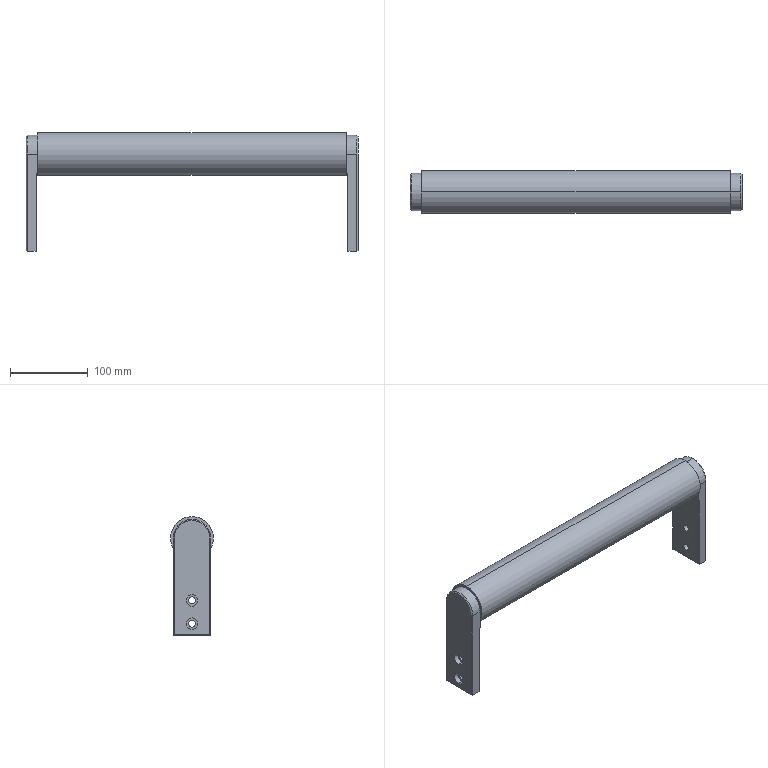Part | SolidWorks | features ICE 2, Chamfer 1, Extrusion 1, HoleWzd 1, MirrorPattern 1 | 1 solid | 54 faces | box 426 x 55 x 152.5 mm | volume 1121917 mm3 | plane 30 | cylinder 21 | cone 3 | commonest cylinder face diameters 9 x8 15 x8 48 x3 55 x2
STEP:
#1=CARTESIAN_POINT('',(-405.,0.,-25.));
#2=VERTEX_POINT('',#1);
#3=CARTESIAN_POINT('',(-405.,0.,-10.));
#4=VERTEX_POINT('',#3);
#5=CARTESIAN_POINT('',(-405.,0.,-17.5));
#6=DIRECTION('',(-1.,0.,0.));
#7=DIRECTION('',(0.,0.,1.));
#8=AXIS2_PLACEMENT_3D('',#5,#6,#7);
#9=CIRCLE('',#8,7.5);
#10=EDGE_CURVE('',#2,#4,#9,.T.);
#11=ORIENTED_EDGE('',*,*,#10,.F.);
#12=CARTESIAN_POINT('',(-411.,0.,-25.));
#13=VERTEX_POINT('',#12);
#14=CARTESIAN_POINT('',(-411.,0.,-25.));
#15=DIRECTION('',(-1.,0.,0.));
#16=VECTOR('',#15,1000.);
#17=LINE('',#14,#16);
#18=EDGE_CURVE('',#2,#13,#17,.T.);
#19=ORIENTED_EDGE('',*,*,#18,.T.);
#20=CARTESIAN_POINT('',(-411.,0.,-10.));
#21=VERTEX_POINT('',#20);
#22=CARTESIAN_POINT('',(-411.,0.,-17.5));
#23=DIRECTION('',(-1.,0.,0.));
#24=DIRECTION('',(0.,0.,1.));
#25=AXIS2_PLACEMENT_3D('',#22,#23,#24);
#26=CIRCLE('',#25,7.5);
#27=EDGE_CURVE('',#13,#21,#26,.T.);
#28=ORIENTED_EDGE('',*,*,#27,.T.);
#29=CARTESIAN_POINT('',(-411.,0.,-10.));
#30=DIRECTION('',(-1.,0.,0.));
#31=VECTOR('',#30,1000.);
#32=LINE('',#29,#31);
#33=EDGE_CURVE('',#4,#21,#32,.T.);
#34=ORIENTED_EDGE('',*,*,#33,.F.);
#35=EDGE_LOOP('',(#11,#19,#28,#34));
#36=FACE_OUTER_BOUND('',#35,.T.);
#37=CARTESIAN_POINT('',(-411.,0.,-17.5));
#38=DIRECTION('',(-1.,0.,0.));
#39=DIRECTION('',(0.,0.,1.));
#40=AXIS2_PLACEMENT_3D('',#37,#38,#39);
#41=CYLINDRICAL_SURFACE('',#40,7.5);
#42=ADVANCED_FACE('',(#36),#41,.F.);
#43=CARTESIAN_POINT('',(-398.,0.,-13.));
#44=VERTEX_POINT('',#43);
#45=CARTESIAN_POINT('',(-398.,0.,-22.));
#46=VERTEX_POINT('',#45);
#47=CARTESIAN_POINT('',(-398.,0.,-17.5));
#48=DIRECTION('',(1.,0.,0.));
#49=DIRECTION('',(0.,0.,1.));
#50=AXIS2_PLACEMENT_3D('',#47,#48,#49);
#51=CIRCLE('',#50,4.5);
#52=EDGE_CURVE('',#44,#46,#51,.T.);
#53=ORIENTED_EDGE('',*,*,#52,.T.);
#54=CARTESIAN_POINT('',(-405.,0.,-22.));
#55=VERTEX_POINT('',#54);
#56=CARTESIAN_POINT('',(-411.,0.,-22.));
#57=DIRECTION('',(-1.,0.,0.));
#58=VECTOR('',#57,1000.);
#59=LINE('',#56,#58);
#60=EDGE_CURVE('',#46,#55,#59,.T.);
#61=ORIENTED_EDGE('',*,*,#60,.T.);
#62=CARTESIAN_POINT('',(-405.,0.,-13.));
#63=VERTEX_POINT('',#62);
#64=CARTESIAN_POINT('',(-405.,0.,-17.5));
#65=DIRECTION('',(-1.,0.,0.));
#66=DIRECTION('',(0.,0.,1.));
#67=AXIS2_PLACEMENT_3D('',#64,#65,#66);
#68=CIRCLE('',#67,4.5);
#69=EDGE_CURVE('',#55,#63,#68,.T.);
#70=ORIENTED_EDGE('',*,*,#69,.T.);
#71=CARTESIAN_POINT('',(-411.,0.,-13.));
#72=DIRECTION('',(-1.,0.,0.));
#73=VECTOR('',#72,1000.);
#74=LINE('',#71,#73);
#75=EDGE_CURVE('',#44,#63,#74,.T.);
#76=ORIENTED_EDGE('',*,*,#75,.F.);
#77=EDGE_LOOP('',(#53,#61,#70,#76));
#78=FACE_OUTER_BOUND('',#77,.T.);
#79=CARTESIAN_POINT('',(-411.,0.,-17.5));
#80=DIRECTION('',(-1.,0.,0.));
#81=DIRECTION('',(0.,0.,1.));
#82=AXIS2_PLACEMENT_3D('',#79,#80,#81);
#83=CYLINDRICAL_SURFACE('',#82,4.5);
#84=ADVANCED_FACE('',(#78),#83,.F.);
#85=CARTESIAN_POINT('',(-405.,0.,-55.));
#86=VERTEX_POINT('',#85);
#87=CARTESIAN_POINT('',(-405.,0.,-40.));
#88=VERTEX_POINT('',#87);
#89=CARTESIAN_POINT('',(-405.,0.,-47.5));
#90=DIRECTION('',(-1.,0.,0.));
#91=DIRECTION('',(0.,0.,1.));
#92=AXIS2_PLACEMENT_3D('',#89,#90,#91);
#93=CIRCLE('',#92,7.5);
#94=EDGE_CURVE('',#86,#88,#93,.T.);
#95=ORIENTED_EDGE('',*,*,#94,.F.);
#96=CARTESIAN_POINT('',(-411.,0.,-55.));
#97=VERTEX_POINT('',#96);
#98=CARTESIAN_POINT('',(-411.,0.,-55.));
#99=DIRECTION('',(-1.,0.,0.));
#100=VECTOR('',#99,1000.);
#101=LINE('',#98,#100);
#102=EDGE_CURVE('',#86,#97,#101,.T.);
#103=ORIENTED_EDGE('',*,*,#102,.T.);
#104=CARTESIAN_POINT('',(-411.,0.,-40.));
#105=VERTEX_POINT('',#104);
#106=CARTESIAN_POINT('',(-411.,0.,-47.5));
#107=DIRECTION('',(-1.,0.,0.));
#108=DIRECTION('',(0.,0.,1.));
#109=AXIS2_PLACEMENT_3D('',#106,#107,#108);
#110=CIRCLE('',#109,7.5);
#111=EDGE_CURVE('',#97,#105,#110,.T.);
#112=ORIENTED_EDGE('',*,*,#111,.T.);
#113=CARTESIAN_POINT('',(-411.,0.,-40.));
#114=DIRECTION('',(-1.,0.,0.));
#115=VECTOR('',#114,1000.);
#116=LINE('',#113,#115);
#117=EDGE_CURVE('',#88,#105,#116,.T.);
#118=ORIENTED_EDGE('',*,*,#117,.F.);
#119=EDGE_LOOP('',(#95,#103,#112,#118));
#120=FACE_OUTER_BOUND('',#119,.T.);
#121=CARTESIAN_POINT('',(-411.,0.,-47.5));
#122=DIRECTION('',(-1.,0.,0.));
#123=DIRECTION('',(0.,0.,1.));
#124=AXIS2_PLACEMENT_3D('',#121,#122,#123);
#125=CYLINDRICAL_SURFACE('',#124,7.5);
#126=ADVANCED_FACE('',(#120),#125,.F.);
#127=CARTESIAN_POINT('',(-398.,0.,-43.));
#128=VERTEX_POINT('',#127);
#129=CARTESIAN_POINT('',(-398.,0.,-52.));
#130=VERTEX_POINT('',#129);
#131=CARTESIAN_POINT('',(-398.,0.,-47.5));
#132=DIRECTION('',(1.,0.,0.));
#133=DIRECTION('',(0.,0.,1.));
#134=AXIS2_PLACEMENT_3D('',#131,#132,#133);
#135=CIRCLE('',#134,4.5);
#136=EDGE_CURVE('',#128,#130,#135,.T.);
#137=ORIENTED_EDGE('',*,*,#136,.T.);
#138=CARTESIAN_POINT('',(-405.,0.,-52.));
#139=VERTEX_POINT('',#138);
#140=CARTESIAN_POINT('',(-411.,0.,-52.));
#141=DIRECTION('',(-1.,0.,0.));
#142=VECTOR('',#141,1000.);
#143=LINE('',#140,#142);
#144=EDGE_CURVE('',#130,#139,#143,.T.);
#145=ORIENTED_EDGE('',*,*,#144,.T.);
#146=CARTESIAN_POINT('',(-405.,0.,-43.));
#147=VERTEX_POINT('',#146);
#148=CARTESIAN_POINT('',(-405.,0.,-47.5));
#149=DIRECTION('',(-1.,0.,0.));
#150=DIRECTION('',(0.,0.,1.));
#151=AXIS2_PLACEMENT_3D('',#148,#149,#150);
#152=CIRCLE('',#151,4.5);
#153=EDGE_CURVE('',#139,#147,#152,.T.);
#154=ORIENTED_EDGE('',*,*,#153,.T.);
#155=CARTESIAN_POINT('',(-411.,0.,-43.));
#156=DIRECTION('',(-1.,0.,0.));
#157=VECTOR('',#156,1000.);
#158=LINE('',#155,#157);
#159=EDGE_CURVE('',#128,#147,#158,.T.);
#160=ORIENTED_EDGE('',*,*,#159,.F.);
#161=EDGE_LOOP('',(#137,#145,#154,#160));
#162=FACE_OUTER_BOUND('',#161,.T.);
#163=CARTESIAN_POINT('',(-411.,0.,-47.5));
#164=DIRECTION('',(-1.,0.,0.));
#165=DIRECTION('',(0.,0.,1.));
#166=AXIS2_PLACEMENT_3D('',#163,#164,#165);
#167=CYLINDRICAL_SURFACE('',#166,4.5);
#168=ADVANCED_FACE('',(#162),#167,.F.);
#169=CARTESIAN_POINT('',(15.,0.,85.));
#170=VERTEX_POINT('',#169);
#171=CARTESIAN_POINT('',(15.,-22.5,62.5));
#172=VERTEX_POINT('',#171);
#173=CARTESIAN_POINT('',(15.,0.,62.5));
#174=DIRECTION('',(1.,0.,0.));
#175=DIRECTION('',(0.,0.,-1.));
#176=AXIS2_PLACEMENT_3D('',#173,#174,#175);
#177=CIRCLE('',#176,22.5);
#178=EDGE_CURVE('',#170,#172,#177,.T.);
#179=ORIENTED_EDGE('',*,*,#178,.F.);
#180=CARTESIAN_POINT('',(13.5,0.,86.5));
#181=VERTEX_POINT('',#180);
#182=CARTESIAN_POINT('',(15.,0.,85.));
#183=DIRECTION('',(-0.7071,0.,0.7071));
#184=VECTOR('',#183,1000.);
#185=LINE('',#182,#184);
#186=EDGE_CURVE('',#170,#181,#185,.T.);
#187=ORIENTED_EDGE('',*,*,#186,.T.);
#188=CARTESIAN_POINT('',(13.5,-24.,62.5));
#189=VERTEX_POINT('',#188);
#190=CARTESIAN_POINT('',(13.5,0.,62.5));
#191=DIRECTION('',(-1.,0.,0.));
#192=DIRECTION('',(0.,0.,-1.));
#193=AXIS2_PLACEMENT_3D('',#190,#191,#192);
#194=CIRCLE('',#193,24.);
#195=EDGE_CURVE('',#189,#181,#194,.T.);
#196=ORIENTED_EDGE('',*,*,#195,.F.);
#197=CARTESIAN_POINT('',(15.,-22.5,62.5));
#198=DIRECTION('',(-0.7071,-0.7071,0.));
#199=VECTOR('',#198,1000.);
#200=LINE('',#197,#199);
#201=EDGE_CURVE('',#172,#189,#200,.T.);
#202=ORIENTED_EDGE('',*,*,#201,.F.);
#203=EDGE_LOOP('',(#179,#187,#196,#202));
#204=FACE_OUTER_BOUND('',#203,.T.);
#205=CARTESIAN_POINT('',(15.,0.,62.5));
#206=DIRECTION('',(-1.,0.,0.));
#207=DIRECTION('',(0.,0.,1.));
#208=AXIS2_PLACEMENT_3D('',#205,#206,#207);
#209=CONICAL_SURFACE('',#208,22.5,0.7854);
#210=ADVANCED_FACE('',(#204),#209,.T.);
#211=CARTESIAN_POINT('',(9.,0.,-10.));
#212=VERTEX_POINT('',#211);
#213=CARTESIAN_POINT('',(9.,0.,-25.));
#214=VERTEX_POINT('',#213);
#215=CARTESIAN_POINT('',(9.,0.,-17.5));
#216=DIRECTION('',(1.,0.,0.));
#217=DIRECTION('',(0.,0.,-1.));
#218=AXIS2_PLACEMENT_3D('',#215,#216,#217);
#219=CIRCLE('',#218,7.5);
#220=EDGE_CURVE('',#212,#214,#219,.T.);
#221=ORIENTED_EDGE('',*,*,#220,.F.);
#222=CARTESIAN_POINT('',(15.,0.,-10.));
#223=VERTEX_POINT('',#222);
#224=CARTESIAN_POINT('',(15.,0.,-10.));
#225=DIRECTION('',(1.,0.,0.));
#226=VECTOR('',#225,1000.);
#227=LINE('',#224,#226);
#228=EDGE_CURVE('',#212,#223,#227,.T.);
#229=ORIENTED_EDGE('',*,*,#228,.T.);
#230=CARTESIAN_POINT('',(15.,0.,-25.));
#231=VERTEX_POINT('',#230);
#232=CARTESIAN_POINT('',(15.,0.,-17.5));
#233=DIRECTION('',(1.,0.,0.));
#234=DIRECTION('',(0.,0.,-1.));
#235=AXIS2_PLACEMENT_3D('',#232,#233,#234);
#236=CIRCLE('',#235,7.5);
#237=EDGE_CURVE('',#223,#231,#236,.T.);
#238=ORIENTED_EDGE('',*,*,#237,.T.);
#239=CARTESIAN_POINT('',(15.,0.,-25.));
#240=DIRECTION('',(1.,0.,0.));
#241=VECTOR('',#240,1000.);
#242=LINE('',#239,#241);
#243=EDGE_CURVE('',#214,#231,#242,.T.);
#244=ORIENTED_EDGE('',*,*,#243,.F.);
#245=EDGE_LOOP('',(#221,#229,#238,#244));
#246=FACE_OUTER_BOUND('',#245,.T.);
#247=CARTESIAN_POINT('',(15.,0.,-17.5));
#248=DIRECTION('',(1.,0.,0.));
#249=DIRECTION('',(0.,0.,-1.));
#250=AXIS2_PLACEMENT_3D('',#247,#248,#249);
#251=CYLINDRICAL_SURFACE('',#250,7.5);
#252=ADVANCED_FACE('',(#246),#251,.F.);
#253=CARTESIAN_POINT('',(2.,0.,-22.));
#254=VERTEX_POINT('',#253);
#255=CARTESIAN_POINT('',(2.,0.,-13.));
#256=VERTEX_POINT('',#255);
#257=CARTESIAN_POINT('',(2.,0.,-17.5));
#258=DIRECTION('',(-1.,0.,0.));
#259=DIRECTION('',(0.,0.,-1.));
#260=AXIS2_PLACEMENT_3D('',#257,#258,#259);
#261=CIRCLE('',#260,4.5);
#262=EDGE_CURVE('',#254,#256,#261,.T.);
#263=ORIENTED_EDGE('',*,*,#262,.T.);
#264=CARTESIAN_POINT('',(9.,0.,-13.));
#265=VERTEX_POINT('',#264);
#266=CARTESIAN_POINT('',(15.,0.,-13.));
#267=DIRECTION('',(1.,0.,0.));
#268=VECTOR('',#267,1000.);
#269=LINE('',#266,#268);
#270=EDGE_CURVE('',#256,#265,#269,.T.);
#271=ORIENTED_EDGE('',*,*,#270,.T.);
#272=CARTESIAN_POINT('',(9.,0.,-22.));
#273=VERTEX_POINT('',#272);
#274=CARTESIAN_POINT('',(9.,0.,-17.5));
#275=DIRECTION('',(1.,0.,0.));
#276=DIRECTION('',(0.,0.,-1.));
#277=AXIS2_PLACEMENT_3D('',#274,#275,#276);
#278=CIRCLE('',#277,4.5);
#279=EDGE_CURVE('',#265,#273,#278,.T.);
#280=ORIENTED_EDGE('',*,*,#279,.T.);
#281=CARTESIAN_POINT('',(15.,0.,-22.));
#282=DIRECTION('',(1.,0.,0.));
#283=VECTOR('',#282,1000.);
#284=LINE('',#281,#283);
#285=EDGE_CURVE('',#254,#273,#284,.T.);
#286=ORIENTED_EDGE('',*,*,#285,.F.);
#287=EDGE_LOOP('',(#263,#271,#280,#286));
#288=FACE_OUTER_BOUND('',#287,.T.);
#289=CARTESIAN_POINT('',(15.,0.,-17.5));
#290=DIRECTION('',(1.,0.,0.));
#291=DIRECTION('',(0.,0.,-1.));
#292=AXIS2_PLACEMENT_3D('',#289,#290,#291);
#293=CYLINDRICAL_SURFACE('',#292,4.5);
#294=ADVANCED_FACE('',(#288),#293,.F.);
#295=CARTESIAN_POINT('',(9.,0.,-40.));
#296=VERTEX_POINT('',#295);
#297=CARTESIAN_POINT('',(9.,0.,-55.));
#298=VERTEX_POINT('',#297);
#299=CARTESIAN_POINT('',(9.,0.,-47.5));
#300=DIRECTION('',(1.,0.,0.));
#301=DIRECTION('',(0.,0.,-1.));
#302=AXIS2_PLACEMENT_3D('',#299,#300,#301);
#303=CIRCLE('',#302,7.5);
#304=EDGE_CURVE('',#296,#298,#303,.T.);
#305=ORIENTED_EDGE('',*,*,#304,.F.);
#306=CARTESIAN_POINT('',(15.,0.,-40.));
#307=VERTEX_POINT('',#306);
#308=CARTESIAN_POINT('',(15.,0.,-40.));
#309=DIRECTION('',(1.,0.,0.));
#310=VECTOR('',#309,1000.);
#311=LINE('',#308,#310);
#312=EDGE_CURVE('',#296,#307,#311,.T.);
#313=ORIENTED_EDGE('',*,*,#312,.T.);
#314=CARTESIAN_POINT('',(15.,0.,-55.));
#315=VERTEX_POINT('',#314);
#316=CARTESIAN_POINT('',(15.,0.,-47.5));
#317=DIRECTION('',(1.,0.,0.));
#318=DIRECTION('',(0.,0.,-1.));
#319=AXIS2_PLACEMENT_3D('',#316,#317,#318);
#320=CIRCLE('',#319,7.5);
#321=EDGE_CURVE('',#307,#315,#320,.T.);
#322=ORIENTED_EDGE('',*,*,#321,.T.);
#323=CARTESIAN_POINT('',(15.,0.,-55.));
#324=DIRECTION('',(1.,0.,0.));
#325=VECTOR('',#324,1000.);
#326=LINE('',#323,#325);
#327=EDGE_CURVE('',#298,#315,#326,.T.);
#328=ORIENTED_EDGE('',*,*,#327,.F.);
#329=EDGE_LOOP('',(#305,#313,#322,#328));
#330=FACE_OUTER_BOUND('',#329,.T.);
#331=CARTESIAN_POINT('',(15.,0.,-47.5));
#332=DIRECTION('',(1.,0.,0.));
#333=DIRECTION('',(0.,0.,-1.));
#334=AXIS2_PLACEMENT_3D('',#331,#332,#333);
#335=CYLINDRICAL_SURFACE('',#334,7.5);
#336=ADVANCED_FACE('',(#330),#335,.F.);
#337=CARTESIAN_POINT('',(2.,0.,-52.));
#338=VERTEX_POINT('',#337);
#339=CARTESIAN_POINT('',(2.,0.,-43.));
#340=VERTEX_POINT('',#339);
#341=CARTESIAN_POINT('',(2.,0.,-47.5));
#342=DIRECTION('',(-1.,0.,0.));
#343=DIRECTION('',(0.,0.,-1.));
#344=AXIS2_PLACEMENT_3D('',#341,#342,#343);
#345=CIRCLE('',#344,4.5);
#346=EDGE_CURVE('',#338,#340,#345,.T.);
#347=ORIENTED_EDGE('',*,*,#346,.T.);
#348=CARTESIAN_POINT('',(9.,0.,-43.));
#349=VERTEX_POINT('',#348);
#350=CARTESIAN_POINT('',(15.,0.,-43.));
#351=DIRECTION('',(1.,0.,0.));
#352=VECTOR('',#351,1000.);
#353=LINE('',#350,#352);
#354=EDGE_CURVE('',#340,#349,#353,.T.);
#355=ORIENTED_EDGE('',*,*,#354,.T.);
#356=CARTESIAN_POINT('',(9.,0.,-52.));
#357=VERTEX_POINT('',#356);
#358=CARTESIAN_POINT('',(9.,0.,-47.5));
#359=DIRECTION('',(1.,0.,0.));
#360=DIRECTION('',(0.,0.,-1.));
#361=AXIS2_PLACEMENT_3D('',#358,#359,#360);
#362=CIRCLE('',#361,4.5);
#363=EDGE_CURVE('',#349,#357,#362,.T.);
#364=ORIENTED_EDGE('',*,*,#363,.T.);
#365=CARTESIAN_POINT('',(15.,0.,-52.));
#366=DIRECTION('',(1.,0.,0.));
#367=VECTOR('',#366,1000.);
#368=LINE('',#365,#367);
#369=EDGE_CURVE('',#338,#357,#368,.T.);
#370=ORIENTED_EDGE('',*,*,#369,.F.);
#371=EDGE_LOOP('',(#347,#355,#364,#370));
#372=FACE_OUTER_BOUND('',#371,.T.);
#373=CARTESIAN_POINT('',(15.,0.,-47.5));
#374=DIRECTION('',(1.,0.,0.));
#375=DIRECTION('',(0.,0.,-1.));
#376=AXIS2_PLACEMENT_3D('',#373,#374,#375);
#377=CYLINDRICAL_SURFACE('',#376,4.5);
#378=ADVANCED_FACE('',(#372),#377,.F.);
#379=CARTESIAN_POINT('',(-396.,0.,90.));
#380=VERTEX_POINT('',#379);
#381=CARTESIAN_POINT('',(-396.,24.,49.074));
#382=VERTEX_POINT('',#381);
#383=CARTESIAN_POINT('',(-396.,0.,62.5));
#384=DIRECTION('',(-1.,0.,0.));
#385=DIRECTION('',(0.,0.,1.));
#386=AXIS2_PLACEMENT_3D('',#383,#384,#385);
#387=CIRCLE('',#386,27.5);
#388=EDGE_CURVE('',#380,#382,#387,.T.);
#389=ORIENTED_EDGE('',*,*,#388,.F.);
#390=CARTESIAN_POINT('',(0.,0.,90.));
#391=VERTEX_POINT('',#390);
#392=CARTESIAN_POINT('',(-396.,0.,90.));
#393=DIRECTION('',(1.,0.,0.));
#394=VECTOR('',#393,1000.);
#395=LINE('',#392,#394);
#396=EDGE_CURVE('',#380,#391,#395,.T.);
#397=ORIENTED_EDGE('',*,*,#396,.T.);
#398=CARTESIAN_POINT('',(0.,24.,49.074));
#399=VERTEX_POINT('',#398);
#400=CARTESIAN_POINT('',(0.,0.,62.5));
#401=DIRECTION('',(-1.,0.,0.));
#402=DIRECTION('',(0.,0.,1.));
#403=AXIS2_PLACEMENT_3D('',#400,#401,#402);
#404=CIRCLE('',#403,27.5);
#405=EDGE_CURVE('',#391,#399,#404,.T.);
#406=ORIENTED_EDGE('',*,*,#405,.T.);
#407=CARTESIAN_POINT('',(0.,11.456,37.5));
#408=VERTEX_POINT('',#407);
#409=CARTESIAN_POINT('',(0.,0.,62.5));
#410=DIRECTION('',(-1.,0.,0.));
#411=DIRECTION('',(0.,0.,1.));
#412=AXIS2_PLACEMENT_3D('',#409,#410,#411);
#413=CIRCLE('',#412,27.5);
#414=EDGE_CURVE('',#399,#408,#413,.T.);
#415=ORIENTED_EDGE('',*,*,#414,.T.);
#416=CARTESIAN_POINT('',(0.,0.,35.));
#417=VERTEX_POINT('',#416);
#418=CARTESIAN_POINT('',(0.,0.,62.5));
#419=DIRECTION('',(-1.,0.,0.));
#420=DIRECTION('',(0.,0.,1.));
#421=AXIS2_PLACEMENT_3D('',#418,#419,#420);
#422=CIRCLE('',#421,27.5);
#423=EDGE_CURVE('',#408,#417,#422,.T.);
#424=ORIENTED_EDGE('',*,*,#423,.T.);
#425=CARTESIAN_POINT('',(-396.,0.,35.));
#426=VERTEX_POINT('',#425);
#427=CARTESIAN_POINT('',(-396.,0.,35.));
#428=DIRECTION('',(1.,0.,0.));
#429=VECTOR('',#428,1000.);
#430=LINE('',#427,#429);
#431=EDGE_CURVE('',#426,#417,#430,.T.);
#432=ORIENTED_EDGE('',*,*,#431,.F.);
#433=CARTESIAN_POINT('',(-396.,11.456,37.5));
#434=VERTEX_POINT('',#433);
#435=CARTESIAN_POINT('',(-396.,0.,62.5));
#436=DIRECTION('',(1.,0.,0.));
#437=DIRECTION('',(0.,0.,-1.));
#438=AXIS2_PLACEMENT_3D('',#435,#436,#437);
#439=CIRCLE('',#438,27.5);
#440=EDGE_CURVE('',#426,#434,#439,.T.);
#441=ORIENTED_EDGE('',*,*,#440,.T.);
#442=CARTESIAN_POINT('',(-396.,0.,62.5));
#443=DIRECTION('',(-1.,0.,0.));
#444=DIRECTION('',(0.,0.,1.));
#445=AXIS2_PLACEMENT_3D('',#442,#443,#444);
#446=CIRCLE('',#445,27.5);
#447=EDGE_CURVE('',#382,#434,#446,.T.);
#448=ORIENTED_EDGE('',*,*,#447,.F.);
#449=EDGE_LOOP('',(#389,#397,#406,#415,#424,#432,#441,#448));
#450=FACE_OUTER_BOUND('',#449,.T.);
#451=CARTESIAN_POINT('',(-396.,0.,62.5));
#452=DIRECTION('',(1.,0.,0.));
#453=DIRECTION('',(0.,0.,-1.));
#454=AXIS2_PLACEMENT_3D('',#451,#452,#453);
#455=CYLINDRICAL_SURFACE('',#454,27.5);
#456=ADVANCED_FACE('',(#450),#455,.T.);
#457=ORIENTED_EDGE('',*,*,#195,.T.);
#458=CARTESIAN_POINT('',(0.,0.,86.5));
#459=VERTEX_POINT('',#458);
#460=CARTESIAN_POINT('',(15.,0.,86.5));
#461=DIRECTION('',(-1.,0.,0.));
#462=VECTOR('',#461,1000.);
#463=LINE('',#460,#462);
#464=EDGE_CURVE('',#181,#459,#463,.T.);
#465=ORIENTED_EDGE('',*,*,#464,.T.);
#466=CARTESIAN_POINT('',(0.,-24.,62.5));
#467=VERTEX_POINT('',#466);
#468=CARTESIAN_POINT('',(0.,0.,62.5));
#469=DIRECTION('',(1.,0.,0.));
#470=DIRECTION('',(0.,0.,-1.));
#471=AXIS2_PLACEMENT_3D('',#468,#469,#470);
#472=CIRCLE('',#471,24.);
#473=EDGE_CURVE('',#459,#467,#472,.T.);
#474=ORIENTED_EDGE('',*,*,#473,.T.);
#475=CARTESIAN_POINT('',(15.,-24.,62.5));
#476=DIRECTION('',(-1.,0.,0.));
#477=VECTOR('',#476,1000.);
#478=LINE('',#475,#477);
#479=EDGE_CURVE('',#189,#467,#478,.T.);
#480=ORIENTED_EDGE('',*,*,#479,.F.);
#481=EDGE_LOOP('',(#457,#465,#474,#480));
#482=FACE_OUTER_BOUND('',#481,.T.);
#483=CARTESIAN_POINT('',(15.,0.,62.5));
#484=DIRECTION('',(-1.,0.,0.));
#485=DIRECTION('',(0.,0.,1.));
#486=AXIS2_PLACEMENT_3D('',#483,#484,#485);
#487=CYLINDRICAL_SURFACE('',#486,24.);
#488=ADVANCED_FACE('',(#482),#487,.T.);
#489=CARTESIAN_POINT('',(0.,24.,37.5));
#490=VERTEX_POINT('',#489);
#491=CARTESIAN_POINT('',(0.,24.,62.5));
#492=DIRECTION('',(0.,0.,1.));
#493=VECTOR('',#492,1000.);
#494=LINE('',#491,#493);
#495=EDGE_CURVE('',#490,#399,#494,.T.);
#496=ORIENTED_EDGE('',*,*,#495,.F.);
#497=CARTESIAN_POINT('',(0.,-27.5,37.5));
#498=DIRECTION('',(0.,1.,0.));
#499=VECTOR('',#498,1000.);
#500=LINE('',#497,#499);
#501=EDGE_CURVE('',#408,#490,#500,.T.);
#502=ORIENTED_EDGE('',*,*,#501,.F.);
#503=ORIENTED_EDGE('',*,*,#414,.F.);
#504=EDGE_LOOP('',(#496,#502,#503));
#505=FACE_OUTER_BOUND('',#504,.T.);
#506=CARTESIAN_POINT('',(0.,0.,62.5));
#507=DIRECTION('',(1.,0.,0.));
#508=DIRECTION('',(0.,0.,-1.));
#509=AXIS2_PLACEMENT_3D('',#506,#507,#508);
#510=PLANE('',#509);
#511=ADVANCED_FACE('',(#505),#510,.F.);
#512=CARTESIAN_POINT('',(-396.,-24.,49.074));
#513=VERTEX_POINT('',#512);
#514=CARTESIAN_POINT('',(-396.,-24.,37.5));
#515=VERTEX_POINT('',#514);
#516=CARTESIAN_POINT('',(-396.,-24.,62.5));
#517=DIRECTION('',(0.,0.,-1.));
#518=VECTOR('',#517,1000.);
#519=LINE('',#516,#518);
#520=EDGE_CURVE('',#513,#515,#519,.T.);
#521=ORIENTED_EDGE('',*,*,#520,.T.);
#522=CARTESIAN_POINT('',(-396.,-11.456,37.5));
#523=VERTEX_POINT('',#522);
#524=CARTESIAN_POINT('',(-396.,-27.5,37.5));
#525=DIRECTION('',(0.,1.,0.));
#526=VECTOR('',#525,1000.);
#527=LINE('',#524,#526);
#528=EDGE_CURVE('',#515,#523,#527,.T.);
#529=ORIENTED_EDGE('',*,*,#528,.T.);
#530=CARTESIAN_POINT('',(-396.,0.,62.5));
#531=DIRECTION('',(-1.,0.,0.));
#532=DIRECTION('',(0.,0.,1.));
#533=AXIS2_PLACEMENT_3D('',#530,#531,#532);
#534=CIRCLE('',#533,27.5);
#535=EDGE_CURVE('',#523,#513,#534,.T.);
#536=ORIENTED_EDGE('',*,*,#535,.T.);
#537=EDGE_LOOP('',(#521,#529,#536));
#538=FACE_OUTER_BOUND('',#537,.T.);
#539=CARTESIAN_POINT('',(-396.,0.,62.5));
#540=DIRECTION('',(-1.,0.,0.));
#541=DIRECTION('',(0.,0.,-1.));
#542=AXIS2_PLACEMENT_3D('',#539,#540,#541);
#543=PLANE('',#542);
#544=ADVANCED_FACE('',(#538),#543,.F.);
#545=CARTESIAN_POINT('',(-396.,0.,62.5));
#546=DIRECTION('',(-1.,0.,0.));
#547=DIRECTION('',(0.,0.,1.));
#548=AXIS2_PLACEMENT_3D('',#545,#546,#547);
#549=CIRCLE('',#548,27.5);
#550=EDGE_CURVE('',#513,#380,#549,.T.);
#551=ORIENTED_EDGE('',*,*,#550,.T.);
#552=ORIENTED_EDGE('',*,*,#388,.T.);
#553=CARTESIAN_POINT('',(-396.,24.,62.5));
#554=VERTEX_POINT('',#553);
#555=CARTESIAN_POINT('',(-396.,24.,62.5));
#556=DIRECTION('',(0.,0.,1.));
#557=VECTOR('',#556,1000.);
#558=LINE('',#555,#557);
#559=EDGE_CURVE('',#382,#554,#558,.T.);
#560=ORIENTED_EDGE('',*,*,#559,.T.);
#561=CARTESIAN_POINT('',(-396.,-24.,62.5));
#562=VERTEX_POINT('',#561);
#563=CARTESIAN_POINT('',(-396.,0.,62.5));
#564=DIRECTION('',(1.,0.,0.));
#565=DIRECTION('',(0.,0.,-1.));
#566=AXIS2_PLACEMENT_3D('',#563,#564,#565);
#567=CIRCLE('',#566,24.);
#568=EDGE_CURVE('',#554,#562,#567,.T.);
#569=ORIENTED_EDGE('',*,*,#568,.T.);
#570=CARTESIAN_POINT('',(-396.,-24.,62.5));
#571=DIRECTION('',(0.,0.,-1.));
#572=VECTOR('',#571,1000.);
#573=LINE('',#570,#572);
#574=EDGE_CURVE('',#562,#513,#573,.T.);
#575=ORIENTED_EDGE('',*,*,#574,.T.);
#576=EDGE_LOOP('',(#551,#552,#560,#569,#575));
#577=FACE_OUTER_BOUND('',#576,.T.);
#578=CARTESIAN_POINT('',(-396.,0.,62.5));
#579=DIRECTION('',(-1.,0.,0.));
#580=DIRECTION('',(0.,0.,1.));
#581=AXIS2_PLACEMENT_3D('',#578,#579,#580);
#582=PLANE('',#581);
#583=ADVANCED_FACE('',(#577),#582,.T.);
#584=CARTESIAN_POINT('',(13.5,-24.,-62.5));
#585=VERTEX_POINT('',#584);
#586=CARTESIAN_POINT('',(2.,-24.,-62.5));
#587=VERTEX_POINT('',#586);
#588=CARTESIAN_POINT('',(15.,-24.,-62.5));
#589=DIRECTION('',(-1.,0.,0.));
#590=VECTOR('',#589,1000.);
#591=LINE('',#588,#590);
#592=EDGE_CURVE('',#585,#587,#591,.T.);
#593=ORIENTED_EDGE('',*,*,#592,.T.);
#594=CARTESIAN_POINT('',(2.,24.,-62.5));
#595=VERTEX_POINT('',#594);
#596=CARTESIAN_POINT('',(2.,-27.5,-62.5));
#597=DIRECTION('',(0.,1.,0.));
#598=VECTOR('',#597,1000.);
#599=LINE('',#596,#598);
#600=EDGE_CURVE('',#587,#595,#599,.T.);
#601=ORIENTED_EDGE('',*,*,#600,.T.);
#602=CARTESIAN_POINT('',(13.5,24.,-62.5));
#603=VERTEX_POINT('',#602);
#604=CARTESIAN_POINT('',(15.,24.,-62.5));
#605=DIRECTION('',(-1.,0.,0.));
#606=VECTOR('',#605,1000.);
#607=LINE('',#604,#606);
#608=EDGE_CURVE('',#603,#595,#607,.T.);
#609=ORIENTED_EDGE('',*,*,#608,.F.);
#610=CARTESIAN_POINT('',(13.5,-24.,-62.5));
#611=DIRECTION('',(0.,-1.,0.));
#612=VECTOR('',#611,1000.);
#613=LINE('',#610,#612);
#614=EDGE_CURVE('',#603,#585,#613,.T.);
#615=ORIENTED_EDGE('',*,*,#614,.T.);
#616=EDGE_LOOP('',(#593,#601,#609,#615));
#617=FACE_OUTER_BOUND('',#616,.T.);
#618=CARTESIAN_POINT('',(15.,24.,-62.5));
#619=DIRECTION('',(0.,0.,1.));
#620=DIRECTION('',(1.,0.,0.));
#621=AXIS2_PLACEMENT_3D('',#618,#619,#620);
#622=PLANE('',#621);
#623=ADVANCED_FACE('',(#617),#622,.F.);
#624=ORIENTED_EDGE('',*,*,#608,.T.);
#625=CARTESIAN_POINT('',(2.,24.,37.5));
#626=VERTEX_POINT('',#625);
#627=CARTESIAN_POINT('',(2.,24.,-62.5));
#628=DIRECTION('',(0.,0.,-1.));
#629=VECTOR('',#628,1000.);
#630=LINE('',#627,#629);
#631=EDGE_CURVE('',#626,#595,#630,.T.);
#632=ORIENTED_EDGE('',*,*,#631,.F.);
#633=CARTESIAN_POINT('',(0.,24.,37.5));
#634=DIRECTION('',(1.,0.,0.));
#635=VECTOR('',#634,1000.);
#636=LINE('',#633,#635);
#637=EDGE_CURVE('',#490,#626,#636,.T.);
#638=ORIENTED_EDGE('',*,*,#637,.F.);
#639=ORIENTED_EDGE('',*,*,#495,.T.);
#640=CARTESIAN_POINT('',(0.,24.,62.5));
#641=VERTEX_POINT('',#640);
#642=CARTESIAN_POINT('',(0.,24.,62.5));
#643=DIRECTION('',(0.,0.,1.));
#644=VECTOR('',#643,1000.);
#645=LINE('',#642,#644);
#646=EDGE_CURVE('',#399,#641,#645,.T.);
#647=ORIENTED_EDGE('',*,*,#646,.T.);
#648=CARTESIAN_POINT('',(13.5,24.,62.5));
#649=VERTEX_POINT('',#648);
#650=CARTESIAN_POINT('',(15.,24.,62.5));
#651=DIRECTION('',(-1.,0.,0.));
#652=VECTOR('',#651,1000.);
#653=LINE('',#650,#652);
#654=EDGE_CURVE('',#649,#641,#653,.T.);
#655=ORIENTED_EDGE('',*,*,#654,.F.);
#656=CARTESIAN_POINT('',(13.5,24.,-62.5));
#657=DIRECTION('',(0.,0.,-1.));
#658=VECTOR('',#657,1000.);
#659=LINE('',#656,#658);
#660=EDGE_CURVE('',#649,#603,#659,.T.);
#661=ORIENTED_EDGE('',*,*,#660,.T.);
#662=EDGE_LOOP('',(#624,#632,#638,#639,#647,#655,#661));
#663=FACE_OUTER_BOUND('',#662,.T.);
#664=CARTESIAN_POINT('',(15.,24.,62.5));
#665=DIRECTION('',(0.,-1.,0.));
#666=DIRECTION('',(0.,0.,-1.));
#667=AXIS2_PLACEMENT_3D('',#664,#665,#666);
#668=PLANE('',#667);
#669=ADVANCED_FACE('',(#663),#668,.F.);
#670=ORIENTED_EDGE('',*,*,#464,.F.);
#671=CARTESIAN_POINT('',(13.5,0.,62.5));
#672=DIRECTION('',(-1.,0.,0.));
#673=DIRECTION('',(0.,0.,-1.));
#674=AXIS2_PLACEMENT_3D('',#671,#672,#673);
#675=CIRCLE('',#674,24.);
#676=EDGE_CURVE('',#181,#649,#675,.T.);
#677=ORIENTED_EDGE('',*,*,#676,.T.);
#678=ORIENTED_EDGE('',*,*,#654,.T.);
#679=CARTESIAN_POINT('',(0.,0.,62.5));
#680=DIRECTION('',(1.,0.,0.));
#681=DIRECTION('',(0.,0.,-1.));
#682=AXIS2_PLACEMENT_3D('',#679,#680,#681);
#683=CIRCLE('',#682,24.);
#684=EDGE_CURVE('',#641,#459,#683,.T.);
#685=ORIENTED_EDGE('',*,*,#684,.T.);
#686=EDGE_LOOP('',(#670,#677,#678,#685));
#687=FACE_OUTER_BOUND('',#686,.T.);
#688=CARTESIAN_POINT('',(15.,0.,62.5));
#689=DIRECTION('',(-1.,0.,0.));
#690=DIRECTION('',(0.,0.,1.));
#691=AXIS2_PLACEMENT_3D('',#688,#689,#690);
#692=CYLINDRICAL_SURFACE('',#691,24.);
#693=ADVANCED_FACE('',(#687),#692,.T.);
#694=CARTESIAN_POINT('',(0.,-24.,37.5));
#695=VERTEX_POINT('',#694);
#696=CARTESIAN_POINT('',(2.,-24.,37.5));
#697=VERTEX_POINT('',#696);
#698=CARTESIAN_POINT('',(15.,-24.,37.5));
#699=DIRECTION('',(1.,0.,0.));
#700=VECTOR('',#699,1000.);
#701=LINE('',#698,#700);
#702=EDGE_CURVE('',#695,#697,#701,.T.);
#703=ORIENTED_EDGE('',*,*,#702,.T.);
#704=CARTESIAN_POINT('',(2.,-24.,62.5));
#705=DIRECTION('',(0.,0.,-1.));
#706=VECTOR('',#705,1000.);
#707=LINE('',#704,#706);
#708=EDGE_CURVE('',#697,#587,#707,.T.);
#709=ORIENTED_EDGE('',*,*,#708,.T.);
#710=ORIENTED_EDGE('',*,*,#592,.F.);
#711=CARTESIAN_POINT('',(13.5,-24.,62.5));
#712=DIRECTION('',(0.,0.,1.));
#713=VECTOR('',#712,1000.);
#714=LINE('',#711,#713);
#715=EDGE_CURVE('',#585,#189,#714,.T.);
#716=ORIENTED_EDGE('',*,*,#715,.T.);
#717=ORIENTED_EDGE('',*,*,#479,.T.);
#718=CARTESIAN_POINT('',(0.,-24.,49.074));
#719=VERTEX_POINT('',#718);
#720=CARTESIAN_POINT('',(0.,-24.,62.5));
#721=DIRECTION('',(0.,0.,-1.));
#722=VECTOR('',#721,1000.);
#723=LINE('',#720,#722);
#724=EDGE_CURVE('',#467,#719,#723,.T.);
#725=ORIENTED_EDGE('',*,*,#724,.T.);
#726=CARTESIAN_POINT('',(0.,-24.,62.5));
#727=DIRECTION('',(0.,0.,-1.));
#728=VECTOR('',#727,1000.);
#729=LINE('',#726,#728);
#730=EDGE_CURVE('',#719,#695,#729,.T.);
#731=ORIENTED_EDGE('',*,*,#730,.T.);
#732=EDGE_LOOP('',(#703,#709,#710,#716,#717,#725,#731));
#733=FACE_OUTER_BOUND('',#732,.T.);
#734=CARTESIAN_POINT('',(15.,-24.,62.5));
#735=DIRECTION('',(0.,1.,0.));
#736=DIRECTION('',(0.,0.,1.));
#737=AXIS2_PLACEMENT_3D('',#734,#735,#736);
#738=PLANE('',#737);
#739=ADVANCED_FACE('',(#733),#738,.F.);
#740=CARTESIAN_POINT('',(15.,-22.5,-61.));
#741=VERTEX_POINT('',#740);
#742=CARTESIAN_POINT('',(15.,-22.5,-62.5));
#743=DIRECTION('',(0.,0.,-1.));
#744=VECTOR('',#743,1000.);
#745=LINE('',#742,#744);
#746=EDGE_CURVE('',#172,#741,#745,.T.);
#747=ORIENTED_EDGE('',*,*,#746,.T.);
#748=CARTESIAN_POINT('',(15.,22.5,-61.));
#749=VERTEX_POINT('',#748);
#750=CARTESIAN_POINT('',(15.,24.,-61.));
#751=DIRECTION('',(0.,1.,0.));
#752=VECTOR('',#751,1000.);
#753=LINE('',#750,#752);
#754=EDGE_CURVE('',#741,#749,#753,.T.);
#755=ORIENTED_EDGE('',*,*,#754,.T.);
#756=CARTESIAN_POINT('',(15.,22.5,62.5));
#757=VERTEX_POINT('',#756);
#758=CARTESIAN_POINT('',(15.,22.5,62.5));
#759=DIRECTION('',(0.,0.,1.));
#760=VECTOR('',#759,1000.);
#761=LINE('',#758,#760);
#762=EDGE_CURVE('',#749,#757,#761,.T.);
#763=ORIENTED_EDGE('',*,*,#762,.T.);
#764=CARTESIAN_POINT('',(15.,0.,62.5));
#765=DIRECTION('',(1.,0.,0.));
#766=DIRECTION('',(0.,0.,-1.));
#767=AXIS2_PLACEMENT_3D('',#764,#765,#766);
#768=CIRCLE('',#767,22.5);
#769=EDGE_CURVE('',#757,#170,#768,.T.);
#770=ORIENTED_EDGE('',*,*,#769,.T.);
#771=ORIENTED_EDGE('',*,*,#178,.T.);
#772=EDGE_LOOP('',(#747,#755,#763,#770,#771));
#773=FACE_OUTER_BOUND('',#772,.T.);
#774=CARTESIAN_POINT('',(15.,0.,-17.5));
#775=DIRECTION('',(1.,0.,0.));
#776=DIRECTION('',(0.,0.,-1.));
#777=AXIS2_PLACEMENT_3D('',#774,#775,#776);
#778=CIRCLE('',#777,7.5);
#779=EDGE_CURVE('',#231,#223,#778,.T.);
#780=ORIENTED_EDGE('',*,*,#779,.F.);
#781=ORIENTED_EDGE('',*,*,#237,.F.);
#782=EDGE_LOOP('',(#780,#781));
#783=FACE_BOUND('',#782,.T.);
#784=CARTESIAN_POINT('',(15.,0.,-47.5));
#785=DIRECTION('',(1.,0.,0.));
#786=DIRECTION('',(0.,0.,-1.));
#787=AXIS2_PLACEMENT_3D('',#784,#785,#786);
#788=CIRCLE('',#787,7.5);
#789=EDGE_CURVE('',#315,#307,#788,.T.);
#790=ORIENTED_EDGE('',*,*,#789,.F.);
#791=ORIENTED_EDGE('',*,*,#321,.F.);
#792=EDGE_LOOP('',(#790,#791));
#793=FACE_BOUND('',#792,.T.);
#794=CARTESIAN_POINT('',(15.,0.,62.5));
#795=DIRECTION('',(1.,0.,0.));
#796=DIRECTION('',(0.,0.,-1.));
#797=AXIS2_PLACEMENT_3D('',#794,#795,#796);
#798=PLANE('',#797);
#799=ADVANCED_FACE('',(#773,#783,#793),#798,.T.);
#800=CARTESIAN_POINT('',(0.,-11.456,37.5));
#801=VERTEX_POINT('',#800);
#802=CARTESIAN_POINT('',(0.,0.,62.5));
#803=DIRECTION('',(-1.,0.,0.));
#804=DIRECTION('',(0.,0.,1.));
#805=AXIS2_PLACEMENT_3D('',#802,#803,#804);
#806=CIRCLE('',#805,27.5);
#807=EDGE_CURVE('',#801,#719,#806,.T.);
#808=ORIENTED_EDGE('',*,*,#807,.F.);
#809=CARTESIAN_POINT('',(0.,-27.5,37.5));
#810=DIRECTION('',(0.,1.,0.));
#811=VECTOR('',#810,1000.);
#812=LINE('',#809,#811);
#813=EDGE_CURVE('',#695,#801,#812,.T.);
#814=ORIENTED_EDGE('',*,*,#813,.F.);
#815=ORIENTED_EDGE('',*,*,#730,.F.);
#816=EDGE_LOOP('',(#808,#814,#815));
#817=FACE_OUTER_BOUND('',#816,.T.);
#818=CARTESIAN_POINT('',(0.,0.,62.5));
#819=DIRECTION('',(1.,0.,0.));
#820=DIRECTION('',(0.,0.,-1.));
#821=AXIS2_PLACEMENT_3D('',#818,#819,#820);
#822=PLANE('',#821);
#823=ADVANCED_FACE('',(#817),#822,.F.);
#824=ORIENTED_EDGE('',*,*,#396,.F.);
#825=ORIENTED_EDGE('',*,*,#550,.F.);
#826=ORIENTED_EDGE('',*,*,#535,.F.);
#827=CARTESIAN_POINT('',(-396.,0.,62.5));
#828=DIRECTION('',(1.,0.,0.));
#829=DIRECTION('',(0.,0.,-1.));
#830=AXIS2_PLACEMENT_3D('',#827,#828,#829);
#831=CIRCLE('',#830,27.5);
#832=EDGE_CURVE('',#523,#426,#831,.T.);
#833=ORIENTED_EDGE('',*,*,#832,.T.);
#834=ORIENTED_EDGE('',*,*,#431,.T.);
#835=CARTESIAN_POINT('',(0.,0.,62.5));
#836=DIRECTION('',(-1.,0.,0.));
#837=DIRECTION('',(0.,0.,1.));
#838=AXIS2_PLACEMENT_3D('',#835,#836,#837);
#839=CIRCLE('',#838,27.5);
#840=EDGE_CURVE('',#417,#801,#839,.T.);
#841=ORIENTED_EDGE('',*,*,#840,.T.);
#842=ORIENTED_EDGE('',*,*,#807,.T.);
#843=CARTESIAN_POINT('',(0.,0.,62.5));
#844=DIRECTION('',(-1.,0.,0.));
#845=DIRECTION('',(0.,0.,1.));
#846=AXIS2_PLACEMENT_3D('',#843,#844,#845);
#847=CIRCLE('',#846,27.5);
#848=EDGE_CURVE('',#719,#391,#847,.T.);
#849=ORIENTED_EDGE('',*,*,#848,.T.);
#850=EDGE_LOOP('',(#824,#825,#826,#833,#834,#841,#842,#849));
#851=FACE_OUTER_BOUND('',#850,.T.);
#852=CARTESIAN_POINT('',(-396.,0.,62.5));
#853=DIRECTION('',(1.,0.,0.));
#854=DIRECTION('',(0.,0.,-1.));
#855=AXIS2_PLACEMENT_3D('',#852,#853,#854);
#856=CYLINDRICAL_SURFACE('',#855,27.5);
#857=ADVANCED_FACE('',(#851),#856,.T.);
#858=ORIENTED_EDGE('',*,*,#724,.F.);
#859=ORIENTED_EDGE('',*,*,#473,.F.);
#860=ORIENTED_EDGE('',*,*,#684,.F.);
#861=ORIENTED_EDGE('',*,*,#646,.F.);
#862=ORIENTED_EDGE('',*,*,#405,.F.);
#863=ORIENTED_EDGE('',*,*,#848,.F.);
#864=EDGE_LOOP('',(#858,#859,#860,#861,#862,#863));
#865=FACE_OUTER_BOUND('',#864,.T.);
#866=CARTESIAN_POINT('',(0.,0.,62.5));
#867=DIRECTION('',(-1.,0.,0.));
#868=DIRECTION('',(0.,0.,1.));
#869=AXIS2_PLACEMENT_3D('',#866,#867,#868);
#870=PLANE('',#869);
#871=ADVANCED_FACE('',(#865),#870,.F.);
#872=ORIENTED_EDGE('',*,*,#354,.F.);
#873=CARTESIAN_POINT('',(2.,0.,-47.5));
#874=DIRECTION('',(-1.,0.,0.));
#875=DIRECTION('',(0.,0.,-1.));
#876=AXIS2_PLACEMENT_3D('',#873,#874,#875);
#877=CIRCLE('',#876,4.5);
#878=EDGE_CURVE('',#340,#338,#877,.T.);
#879=ORIENTED_EDGE('',*,*,#878,.T.);
#880=ORIENTED_EDGE('',*,*,#369,.T.);
#881=CARTESIAN_POINT('',(9.,0.,-47.5));
#882=DIRECTION('',(1.,0.,0.));
#883=DIRECTION('',(0.,0.,-1.));
#884=AXIS2_PLACEMENT_3D('',#881,#882,#883);
#885=CIRCLE('',#884,4.5);
#886=EDGE_CURVE('',#357,#349,#885,.T.);
#887=ORIENTED_EDGE('',*,*,#886,.T.);
#888=EDGE_LOOP('',(#872,#879,#880,#887));
#889=FACE_OUTER_BOUND('',#888,.T.);
#890=CARTESIAN_POINT('',(15.,0.,-47.5));
#891=DIRECTION('',(1.,0.,0.));
#892=DIRECTION('',(0.,0.,-1.));
#893=AXIS2_PLACEMENT_3D('',#890,#891,#892);
#894=CYLINDRICAL_SURFACE('',#893,4.5);
#895=ADVANCED_FACE('',(#889),#894,.F.);
#896=ORIENTED_EDGE('',*,*,#886,.F.);
#897=ORIENTED_EDGE('',*,*,#363,.F.);
#898=EDGE_LOOP('',(#896,#897));
#899=FACE_BOUND('',#898,.T.);
#900=CARTESIAN_POINT('',(9.,0.,-47.5));
#901=DIRECTION('',(1.,0.,0.));
#902=DIRECTION('',(0.,0.,-1.));
#903=AXIS2_PLACEMENT_3D('',#900,#901,#902);
#904=CIRCLE('',#903,7.5);
#905=EDGE_CURVE('',#298,#296,#904,.T.);
#906=ORIENTED_EDGE('',*,*,#905,.T.);
#907=ORIENTED_EDGE('',*,*,#304,.T.);
#908=EDGE_LOOP('',(#906,#907));
#909=FACE_OUTER_BOUND('',#908,.T.);
#910=CARTESIAN_POINT('',(9.,4.5,-47.5));
#911=DIRECTION('',(-1.,0.,0.));
#912=DIRECTION('',(0.,0.,1.));
#913=AXIS2_PLACEMENT_3D('',#910,#911,#912);
#914=PLANE('',#913);
#915=ADVANCED_FACE('',(#899,#909),#914,.F.);
#916=ORIENTED_EDGE('',*,*,#312,.F.);
#917=ORIENTED_EDGE('',*,*,#905,.F.);
#918=ORIENTED_EDGE('',*,*,#327,.T.);
#919=ORIENTED_EDGE('',*,*,#789,.T.);
#920=EDGE_LOOP('',(#916,#917,#918,#919));
#921=FACE_OUTER_BOUND('',#920,.T.);
#922=CARTESIAN_POINT('',(15.,0.,-47.5));
#923=DIRECTION('',(1.,0.,0.));
#924=DIRECTION('',(0.,0.,-1.));
#925=AXIS2_PLACEMENT_3D('',#922,#923,#924);
#926=CYLINDRICAL_SURFACE('',#925,7.5);
#927=ADVANCED_FACE('',(#921),#926,.F.);
#928=ORIENTED_EDGE('',*,*,#270,.F.);
#929=CARTESIAN_POINT('',(2.,0.,-17.5));
#930=DIRECTION('',(-1.,0.,0.));
#931=DIRECTION('',(0.,0.,-1.));
#932=AXIS2_PLACEMENT_3D('',#929,#930,#931);
#933=CIRCLE('',#932,4.5);
#934=EDGE_CURVE('',#256,#254,#933,.T.);
#935=ORIENTED_EDGE('',*,*,#934,.T.);
#936=ORIENTED_EDGE('',*,*,#285,.T.);
#937=CARTESIAN_POINT('',(9.,0.,-17.5));
#938=DIRECTION('',(1.,0.,0.));
#939=DIRECTION('',(0.,0.,-1.));
#940=AXIS2_PLACEMENT_3D('',#937,#938,#939);
#941=CIRCLE('',#940,4.5);
#942=EDGE_CURVE('',#273,#265,#941,.T.);
#943=ORIENTED_EDGE('',*,*,#942,.T.);
#944=EDGE_LOOP('',(#928,#935,#936,#943));
#945=FACE_OUTER_BOUND('',#944,.T.);
#946=CARTESIAN_POINT('',(15.,0.,-17.5));
#947=DIRECTION('',(1.,0.,0.));
#948=DIRECTION('',(0.,0.,-1.));
#949=AXIS2_PLACEMENT_3D('',#946,#947,#948);
#950=CYLINDRICAL_SURFACE('',#949,4.5);
#951=ADVANCED_FACE('',(#945),#950,.F.);
#952=ORIENTED_EDGE('',*,*,#942,.F.);
#953=ORIENTED_EDGE('',*,*,#279,.F.);
#954=EDGE_LOOP('',(#952,#953));
#955=FACE_BOUND('',#954,.T.);
#956=CARTESIAN_POINT('',(9.,0.,-17.5));
#957=DIRECTION('',(1.,0.,0.));
#958=DIRECTION('',(0.,0.,-1.));
#959=AXIS2_PLACEMENT_3D('',#956,#957,#958);
#960=CIRCLE('',#959,7.5);
#961=EDGE_CURVE('',#214,#212,#960,.T.);
#962=ORIENTED_EDGE('',*,*,#961,.T.);
#963=ORIENTED_EDGE('',*,*,#220,.T.);
#964=EDGE_LOOP('',(#962,#963));
#965=FACE_OUTER_BOUND('',#964,.T.);
#966=CARTESIAN_POINT('',(9.,4.5,-17.5));
#967=DIRECTION('',(-1.,0.,0.));
#968=DIRECTION('',(0.,0.,1.));
#969=AXIS2_PLACEMENT_3D('',#966,#967,#968);
#970=PLANE('',#969);
#971=ADVANCED_FACE('',(#955,#965),#970,.F.);
#972=ORIENTED_EDGE('',*,*,#228,.F.);
#973=ORIENTED_EDGE('',*,*,#961,.F.);
#974=ORIENTED_EDGE('',*,*,#243,.T.);
#975=ORIENTED_EDGE('',*,*,#779,.T.);
#976=EDGE_LOOP('',(#972,#973,#974,#975));
#977=FACE_OUTER_BOUND('',#976,.T.);
#978=CARTESIAN_POINT('',(15.,0.,-17.5));
#979=DIRECTION('',(1.,0.,0.));
#980=DIRECTION('',(0.,0.,-1.));
#981=AXIS2_PLACEMENT_3D('',#978,#979,#980);
#982=CYLINDRICAL_SURFACE('',#981,7.5);
#983=ADVANCED_FACE('',(#977),#982,.F.);
#984=ORIENTED_EDGE('',*,*,#186,.F.);
#985=ORIENTED_EDGE('',*,*,#769,.F.);
#986=CARTESIAN_POINT('',(13.5,24.,62.5));
#987=DIRECTION('',(0.7071,-0.7071,0.));
#988=VECTOR('',#987,1000.);
#989=LINE('',#986,#988);
#990=EDGE_CURVE('',#649,#757,#989,.T.);
#991=ORIENTED_EDGE('',*,*,#990,.F.);
#992=ORIENTED_EDGE('',*,*,#676,.F.);
#993=EDGE_LOOP('',(#984,#985,#991,#992));
#994=FACE_OUTER_BOUND('',#993,.T.);
#995=CARTESIAN_POINT('',(15.,0.,62.5));
#996=DIRECTION('',(-1.,0.,0.));
#997=DIRECTION('',(0.,0.,1.));
#998=AXIS2_PLACEMENT_3D('',#995,#996,#997);
#999=CONICAL_SURFACE('',#998,22.5,0.7854);
#1000=ADVANCED_FACE('',(#994),#999,.T.);
#1001=ORIENTED_EDGE('',*,*,#201,.T.);
#1002=ORIENTED_EDGE('',*,*,#715,.F.);
#1003=CARTESIAN_POINT('',(56.167,18.667,-19.833));
#1004=DIRECTION('',(-0.5774,-0.5774,-0.5774));
#1005=VECTOR('',#1004,1000.);
#1006=LINE('',#1003,#1005);
#1007=EDGE_CURVE('',#741,#585,#1006,.T.);
#1008=ORIENTED_EDGE('',*,*,#1007,.F.);
#1009=ORIENTED_EDGE('',*,*,#746,.F.);
#1010=EDGE_LOOP('',(#1001,#1002,#1008,#1009));
#1011=FACE_OUTER_BOUND('',#1010,.T.);
#1012=CARTESIAN_POINT('',(15.,-22.5,62.5));
#1013=DIRECTION('',(0.7071,-0.7071,0.));
#1014=DIRECTION('',(0.,0.,1.));
#1015=AXIS2_PLACEMENT_3D('',#1012,#1013,#1014);
#1016=PLANE('',#1015);
#1017=ADVANCED_FACE('',(#1011),#1016,.T.);
#1018=ORIENTED_EDGE('',*,*,#990,.T.);
#1019=ORIENTED_EDGE('',*,*,#762,.F.);
#1020=CARTESIAN_POINT('',(56.167,-18.667,-19.833));
#1021=DIRECTION('',(0.5774,-0.5774,0.5774));
#1022=VECTOR('',#1021,1000.);
#1023=LINE('',#1020,#1022);
#1024=EDGE_CURVE('',#603,#749,#1023,.T.);
#1025=ORIENTED_EDGE('',*,*,#1024,.F.);
#1026=ORIENTED_EDGE('',*,*,#660,.F.);
#1027=EDGE_LOOP('',(#1018,#1019,#1025,#1026));
#1028=FACE_OUTER_BOUND('',#1027,.T.);
#1029=CARTESIAN_POINT('',(15.,22.5,62.5));
#1030=DIRECTION('',(0.7071,0.7071,0.));
#1031=DIRECTION('',(0.,0.,-1.));
#1032=AXIS2_PLACEMENT_3D('',#1029,#1030,#1031);
#1033=PLANE('',#1032);
#1034=ADVANCED_FACE('',(#1028),#1033,.T.);
#1035=ORIENTED_EDGE('',*,*,#1007,.T.);
#1036=ORIENTED_EDGE('',*,*,#614,.F.);
#1037=ORIENTED_EDGE('',*,*,#1024,.T.);
#1038=ORIENTED_EDGE('',*,*,#754,.F.);
#1039=EDGE_LOOP('',(#1035,#1036,#1037,#1038));
#1040=FACE_OUTER_BOUND('',#1039,.T.);
#1041=CARTESIAN_POINT('',(15.,0.,-61.));
#1042=DIRECTION('',(0.7071,0.,-0.7071));
#1043=DIRECTION('',(0.,-1.,0.));
#1044=AXIS2_PLACEMENT_3D('',#1041,#1042,#1043);
#1045=PLANE('',#1044);
#1046=ADVANCED_FACE('',(#1040),#1045,.T.);
#1047=ORIENTED_EDGE('',*,*,#447,.T.);
#1048=CARTESIAN_POINT('',(-396.,24.,37.5));
#1049=VERTEX_POINT('',#1048);
#1050=CARTESIAN_POINT('',(-396.,-27.5,37.5));
#1051=DIRECTION('',(0.,1.,0.));
#1052=VECTOR('',#1051,1000.);
#1053=LINE('',#1050,#1052);
#1054=EDGE_CURVE('',#434,#1049,#1053,.T.);
#1055=ORIENTED_EDGE('',*,*,#1054,.T.);
#1056=CARTESIAN_POINT('',(-396.,24.,62.5));
#1057=DIRECTION('',(0.,0.,1.));
#1058=VECTOR('',#1057,1000.);
#1059=LINE('',#1056,#1058);
#1060=EDGE_CURVE('',#1049,#382,#1059,.T.);
#1061=ORIENTED_EDGE('',*,*,#1060,.T.);
#1062=EDGE_LOOP('',(#1047,#1055,#1061));
#1063=FACE_OUTER_BOUND('',#1062,.T.);
#1064=CARTESIAN_POINT('',(-396.,0.,62.5));
#1065=DIRECTION('',(-1.,0.,0.));
#1066=DIRECTION('',(0.,0.,-1.));
#1067=AXIS2_PLACEMENT_3D('',#1064,#1065,#1066);
#1068=PLANE('',#1067);
#1069=ADVANCED_FACE('',(#1063),#1068,.F.);
#1070=CARTESIAN_POINT('',(-398.,-24.,-62.5));
#1071=VERTEX_POINT('',#1070);
#1072=CARTESIAN_POINT('',(-398.,24.,-62.5));
#1073=VERTEX_POINT('',#1072);
#1074=CARTESIAN_POINT('',(-398.,-27.5,-62.5));
#1075=DIRECTION('',(0.,1.,0.));
#1076=VECTOR('',#1075,1000.);
#1077=LINE('',#1074,#1076);
#1078=EDGE_CURVE('',#1071,#1073,#1077,.T.);
#1079=ORIENTED_EDGE('',*,*,#1078,.F.);
#1080=CARTESIAN_POINT('',(-409.5,-24.,-62.5));
#1081=VERTEX_POINT('',#1080);
#1082=CARTESIAN_POINT('',(-411.,-24.,-62.5));
#1083=DIRECTION('',(1.,0.,0.));
#1084=VECTOR('',#1083,1000.);
#1085=LINE('',#1082,#1084);
#1086=EDGE_CURVE('',#1081,#1071,#1085,.T.);
#1087=ORIENTED_EDGE('',*,*,#1086,.F.);
#1088=CARTESIAN_POINT('',(-409.5,24.,-62.5));
#1089=VERTEX_POINT('',#1088);
#1090=CARTESIAN_POINT('',(-409.5,24.,-62.5));
#1091=DIRECTION('',(0.,1.,0.));
#1092=VECTOR('',#1091,1000.);
#1093=LINE('',#1090,#1092);
#1094=EDGE_CURVE('',#1081,#1089,#1093,.T.);
#1095=ORIENTED_EDGE('',*,*,#1094,.T.);
#1096=CARTESIAN_POINT('',(-411.,24.,-62.5));
#1097=DIRECTION('',(1.,0.,0.));
#1098=VECTOR('',#1097,1000.);
#1099=LINE('',#1096,#1098);
#1100=EDGE_CURVE('',#1089,#1073,#1099,.T.);
#1101=ORIENTED_EDGE('',*,*,#1100,.T.);
#1102=EDGE_LOOP('',(#1079,#1087,#1095,#1101));
#1103=FACE_OUTER_BOUND('',#1102,.T.);
#1104=CARTESIAN_POINT('',(-411.,24.,-62.5));
#1105=DIRECTION('',(0.,0.,-1.));
#1106=DIRECTION('',(-1.,0.,0.));
#1107=AXIS2_PLACEMENT_3D('',#1104,#1105,#1106);
#1108=PLANE('',#1107);
#1109=ADVANCED_FACE('',(#1103),#1108,.T.);
#1110=CARTESIAN_POINT('',(-398.,-24.,37.5));
#1111=VERTEX_POINT('',#1110);
#1112=CARTESIAN_POINT('',(-411.,-24.,37.5));
#1113=DIRECTION('',(-1.,0.,0.));
#1114=VECTOR('',#1113,1000.);
#1115=LINE('',#1112,#1114);
#1116=EDGE_CURVE('',#515,#1111,#1115,.T.);
#1117=ORIENTED_EDGE('',*,*,#1116,.F.);
#1118=ORIENTED_EDGE('',*,*,#520,.F.);
#1119=ORIENTED_EDGE('',*,*,#574,.F.);
#1120=CARTESIAN_POINT('',(-409.5,-24.,62.5));
#1121=VERTEX_POINT('',#1120);
#1122=CARTESIAN_POINT('',(-411.,-24.,62.5));
#1123=DIRECTION('',(1.,0.,0.));
#1124=VECTOR('',#1123,1000.);
#1125=LINE('',#1122,#1124);
#1126=EDGE_CURVE('',#1121,#562,#1125,.T.);
#1127=ORIENTED_EDGE('',*,*,#1126,.F.);
#1128=CARTESIAN_POINT('',(-409.5,-24.,62.5));
#1129=DIRECTION('',(0.,0.,-1.));
#1130=VECTOR('',#1129,1000.);
#1131=LINE('',#1128,#1130);
#1132=EDGE_CURVE('',#1121,#1081,#1131,.T.);
#1133=ORIENTED_EDGE('',*,*,#1132,.T.);
#1134=ORIENTED_EDGE('',*,*,#1086,.T.);
#1135=CARTESIAN_POINT('',(-398.,-24.,62.5));
#1136=DIRECTION('',(0.,0.,-1.));
#1137=VECTOR('',#1136,1000.);
#1138=LINE('',#1135,#1137);
#1139=EDGE_CURVE('',#1111,#1071,#1138,.T.);
#1140=ORIENTED_EDGE('',*,*,#1139,.F.);
#1141=EDGE_LOOP('',(#1117,#1118,#1119,#1127,#1133,#1134,#1140));
#1142=FACE_OUTER_BOUND('',#1141,.T.);
#1143=CARTESIAN_POINT('',(-411.,-24.,62.5));
#1144=DIRECTION('',(0.,-1.,0.));
#1145=DIRECTION('',(0.,0.,-1.));
#1146=AXIS2_PLACEMENT_3D('',#1143,#1144,#1145);
#1147=PLANE('',#1146);
#1148=ADVANCED_FACE('',(#1142),#1147,.T.);
#1149=CARTESIAN_POINT('',(-409.5,24.,62.5));
#1150=VERTEX_POINT('',#1149);
#1151=CARTESIAN_POINT('',(-411.,24.,62.5));
#1152=DIRECTION('',(1.,0.,0.));
#1153=VECTOR('',#1152,1000.);
#1154=LINE('',#1151,#1153);
#1155=EDGE_CURVE('',#1150,#554,#1154,.T.);
#1156=ORIENTED_EDGE('',*,*,#1155,.F.);
#1157=CARTESIAN_POINT('',(-409.5,0.,62.5));
#1158=DIRECTION('',(1.,0.,0.));
#1159=DIRECTION('',(0.,0.,1.));
#1160=AXIS2_PLACEMENT_3D('',#1157,#1158,#1159);
#1161=CIRCLE('',#1160,24.);
#1162=EDGE_CURVE('',#1150,#1121,#1161,.T.);
#1163=ORIENTED_EDGE('',*,*,#1162,.T.);
#1164=ORIENTED_EDGE('',*,*,#1126,.T.);
#1165=ORIENTED_EDGE('',*,*,#568,.F.);
#1166=EDGE_LOOP('',(#1156,#1163,#1164,#1165));
#1167=FACE_OUTER_BOUND('',#1166,.T.);
#1168=CARTESIAN_POINT('',(-411.,0.,62.5));
#1169=DIRECTION('',(1.,0.,0.));
#1170=DIRECTION('',(0.,0.,-1.));
#1171=AXIS2_PLACEMENT_3D('',#1168,#1169,#1170);
#1172=CYLINDRICAL_SURFACE('',#1171,24.);
#1173=ADVANCED_FACE('',(#1167),#1172,.T.);
#1174=CARTESIAN_POINT('',(-398.,24.,37.5));
#1175=VERTEX_POINT('',#1174);
#1176=CARTESIAN_POINT('',(-396.,24.,37.5));
#1177=DIRECTION('',(1.,0.,0.));
#1178=VECTOR('',#1177,1000.);
#1179=LINE('',#1176,#1178);
#1180=EDGE_CURVE('',#1175,#1049,#1179,.T.);
#1181=ORIENTED_EDGE('',*,*,#1180,.F.);
#1182=CARTESIAN_POINT('',(-398.,24.,-62.5));
#1183=DIRECTION('',(0.,0.,1.));
#1184=VECTOR('',#1183,1000.);
#1185=LINE('',#1182,#1184);
#1186=EDGE_CURVE('',#1073,#1175,#1185,.T.);
#1187=ORIENTED_EDGE('',*,*,#1186,.F.);
#1188=ORIENTED_EDGE('',*,*,#1100,.F.);
#1189=CARTESIAN_POINT('',(-409.5,24.,62.5));
#1190=DIRECTION('',(0.,0.,1.));
#1191=VECTOR('',#1190,1000.);
#1192=LINE('',#1189,#1191);
#1193=EDGE_CURVE('',#1089,#1150,#1192,.T.);
#1194=ORIENTED_EDGE('',*,*,#1193,.T.);
#1195=ORIENTED_EDGE('',*,*,#1155,.T.);
#1196=ORIENTED_EDGE('',*,*,#559,.F.);
#1197=ORIENTED_EDGE('',*,*,#1060,.F.);
#1198=EDGE_LOOP('',(#1181,#1187,#1188,#1194,#1195,#1196,#1197));
#1199=FACE_OUTER_BOUND('',#1198,.T.);
#1200=CARTESIAN_POINT('',(-411.,24.,62.5));
#1201=DIRECTION('',(0.,1.,0.));
#1202=DIRECTION('',(0.,0.,1.));
#1203=AXIS2_PLACEMENT_3D('',#1200,#1201,#1202);
#1204=PLANE('',#1203);
#1205=ADVANCED_FACE('',(#1199),#1204,.T.);
#1206=CARTESIAN_POINT('',(-411.,22.5,62.5));
#1207=VERTEX_POINT('',#1206);
#1208=CARTESIAN_POINT('',(-411.,22.5,-61.));
#1209=VERTEX_POINT('',#1208);
#1210=CARTESIAN_POINT('',(-411.,22.5,62.5));
#1211=DIRECTION('',(0.,0.,-1.));
#1212=VECTOR('',#1211,1000.);
#1213=LINE('',#1210,#1212);
#1214=EDGE_CURVE('',#1207,#1209,#1213,.T.);
#1215=ORIENTED_EDGE('',*,*,#1214,.T.);
#1216=CARTESIAN_POINT('',(-411.,-22.5,-61.));
#1217=VERTEX_POINT('',#1216);
#1218=CARTESIAN_POINT('',(-411.,0.,-61.));
#1219=DIRECTION('',(0.,-1.,0.));
#1220=VECTOR('',#1219,1000.);
#1221=LINE('',#1218,#1220);
#1222=EDGE_CURVE('',#1209,#1217,#1221,.T.);
#1223=ORIENTED_EDGE('',*,*,#1222,.T.);
#1224=CARTESIAN_POINT('',(-411.,-22.5,62.5));
#1225=VERTEX_POINT('',#1224);
#1226=CARTESIAN_POINT('',(-411.,-22.5,62.5));
#1227=DIRECTION('',(0.,0.,1.));
#1228=VECTOR('',#1227,1000.);
#1229=LINE('',#1226,#1228);
#1230=EDGE_CURVE('',#1217,#1225,#1229,.T.);
#1231=ORIENTED_EDGE('',*,*,#1230,.T.);
#1232=CARTESIAN_POINT('',(-411.,0.,62.5));
#1233=DIRECTION('',(-1.,0.,0.));
#1234=DIRECTION('',(0.,0.,1.));
#1235=AXIS2_PLACEMENT_3D('',#1232,#1233,#1234);
#1236=CIRCLE('',#1235,22.5);
#1237=EDGE_CURVE('',#1225,#1207,#1236,.T.);
#1238=ORIENTED_EDGE('',*,*,#1237,.T.);
#1239=EDGE_LOOP('',(#1215,#1223,#1231,#1238));
#1240=FACE_OUTER_BOUND('',#1239,.T.);
#1241=CARTESIAN_POINT('',(-411.,0.,-17.5));
#1242=DIRECTION('',(-1.,0.,0.));
#1243=DIRECTION('',(0.,0.,1.));
#1244=AXIS2_PLACEMENT_3D('',#1241,#1242,#1243);
#1245=CIRCLE('',#1244,7.5);
#1246=EDGE_CURVE('',#21,#13,#1245,.T.);
#1247=ORIENTED_EDGE('',*,*,#1246,.F.);
#1248=ORIENTED_EDGE('',*,*,#27,.F.);
#1249=EDGE_LOOP('',(#1247,#1248));
#1250=FACE_BOUND('',#1249,.T.);
#1251=CARTESIAN_POINT('',(-411.,0.,-47.5));
#1252=DIRECTION('',(-1.,0.,0.));
#1253=DIRECTION('',(0.,0.,1.));
#1254=AXIS2_PLACEMENT_3D('',#1251,#1252,#1253);
#1255=CIRCLE('',#1254,7.5);
#1256=EDGE_CURVE('',#105,#97,#1255,.T.);
#1257=ORIENTED_EDGE('',*,*,#1256,.F.);
#1258=ORIENTED_EDGE('',*,*,#111,.F.);
#1259=EDGE_LOOP('',(#1257,#1258));
#1260=FACE_BOUND('',#1259,.T.);
#1261=CARTESIAN_POINT('',(-411.,0.,62.5));
#1262=DIRECTION('',(-1.,0.,0.));
#1263=DIRECTION('',(0.,0.,-1.));
#1264=AXIS2_PLACEMENT_3D('',#1261,#1262,#1263);
#1265=PLANE('',#1264);
#1266=ADVANCED_FACE('',(#1240,#1250,#1260),#1265,.T.);
#1267=ORIENTED_EDGE('',*,*,#144,.F.);
#1268=CARTESIAN_POINT('',(-398.,0.,-47.5));
#1269=DIRECTION('',(1.,0.,0.));
#1270=DIRECTION('',(0.,0.,1.));
#1271=AXIS2_PLACEMENT_3D('',#1268,#1269,#1270);
#1272=CIRCLE('',#1271,4.5);
#1273=EDGE_CURVE('',#130,#128,#1272,.T.);
#1274=ORIENTED_EDGE('',*,*,#1273,.T.);
#1275=ORIENTED_EDGE('',*,*,#159,.T.);
#1276=CARTESIAN_POINT('',(-405.,0.,-47.5));
#1277=DIRECTION('',(-1.,0.,0.));
#1278=DIRECTION('',(0.,0.,1.));
#1279=AXIS2_PLACEMENT_3D('',#1276,#1277,#1278);
#1280=CIRCLE('',#1279,4.5);
#1281=EDGE_CURVE('',#147,#139,#1280,.T.);
#1282=ORIENTED_EDGE('',*,*,#1281,.T.);
#1283=EDGE_LOOP('',(#1267,#1274,#1275,#1282));
#1284=FACE_OUTER_BOUND('',#1283,.T.);
#1285=CARTESIAN_POINT('',(-411.,0.,-47.5));
#1286=DIRECTION('',(-1.,0.,0.));
#1287=DIRECTION('',(0.,0.,1.));
#1288=AXIS2_PLACEMENT_3D('',#1285,#1286,#1287);
#1289=CYLINDRICAL_SURFACE('',#1288,4.5);
#1290=ADVANCED_FACE('',(#1284),#1289,.F.);
#1291=ORIENTED_EDGE('',*,*,#1281,.F.);
#1292=ORIENTED_EDGE('',*,*,#153,.F.);
#1293=EDGE_LOOP('',(#1291,#1292));
#1294=FACE_BOUND('',#1293,.T.);
#1295=CARTESIAN_POINT('',(-405.,0.,-47.5));
#1296=DIRECTION('',(-1.,0.,0.));
#1297=DIRECTION('',(0.,0.,1.));
#1298=AXIS2_PLACEMENT_3D('',#1295,#1296,#1297);
#1299=CIRCLE('',#1298,7.5);
#1300=EDGE_CURVE('',#88,#86,#1299,.T.);
#1301=ORIENTED_EDGE('',*,*,#1300,.T.);
#1302=ORIENTED_EDGE('',*,*,#94,.T.);
#1303=EDGE_LOOP('',(#1301,#1302));
#1304=FACE_OUTER_BOUND('',#1303,.T.);
#1305=CARTESIAN_POINT('',(-405.,4.5,-47.5));
#1306=DIRECTION('',(1.,0.,0.));
#1307=DIRECTION('',(0.,0.,-1.));
#1308=AXIS2_PLACEMENT_3D('',#1305,#1306,#1307);
#1309=PLANE('',#1308);
#1310=ADVANCED_FACE('',(#1294,#1304),#1309,.F.);
#1311=ORIENTED_EDGE('',*,*,#102,.F.);
#1312=ORIENTED_EDGE('',*,*,#1300,.F.);
#1313=ORIENTED_EDGE('',*,*,#117,.T.);
#1314=ORIENTED_EDGE('',*,*,#1256,.T.);
#1315=EDGE_LOOP('',(#1311,#1312,#1313,#1314));
#1316=FACE_OUTER_BOUND('',#1315,.T.);
#1317=CARTESIAN_POINT('',(-411.,0.,-47.5));
#1318=DIRECTION('',(-1.,0.,0.));
#1319=DIRECTION('',(0.,0.,1.));
#1320=AXIS2_PLACEMENT_3D('',#1317,#1318,#1319);
#1321=CYLINDRICAL_SURFACE('',#1320,7.5);
#1322=ADVANCED_FACE('',(#1316),#1321,.F.);
#1323=ORIENTED_EDGE('',*,*,#60,.F.);
#1324=CARTESIAN_POINT('',(-398.,0.,-17.5));
#1325=DIRECTION('',(1.,0.,0.));
#1326=DIRECTION('',(0.,0.,1.));
#1327=AXIS2_PLACEMENT_3D('',#1324,#1325,#1326);
#1328=CIRCLE('',#1327,4.5);
#1329=EDGE_CURVE('',#46,#44,#1328,.T.);
#1330=ORIENTED_EDGE('',*,*,#1329,.T.);
#1331=ORIENTED_EDGE('',*,*,#75,.T.);
#1332=CARTESIAN_POINT('',(-405.,0.,-17.5));
#1333=DIRECTION('',(-1.,0.,0.));
#1334=DIRECTION('',(0.,0.,1.));
#1335=AXIS2_PLACEMENT_3D('',#1332,#1333,#1334);
#1336=CIRCLE('',#1335,4.5);
#1337=EDGE_CURVE('',#63,#55,#1336,.T.);
#1338=ORIENTED_EDGE('',*,*,#1337,.T.);
#1339=EDGE_LOOP('',(#1323,#1330,#1331,#1338));
#1340=FACE_OUTER_BOUND('',#1339,.T.);
#1341=CARTESIAN_POINT('',(-411.,0.,-17.5));
#1342=DIRECTION('',(-1.,0.,0.));
#1343=DIRECTION('',(0.,0.,1.));
#1344=AXIS2_PLACEMENT_3D('',#1341,#1342,#1343);
#1345=CYLINDRICAL_SURFACE('',#1344,4.5);
#1346=ADVANCED_FACE('',(#1340),#1345,.F.);
#1347=ORIENTED_EDGE('',*,*,#1337,.F.);
#1348=ORIENTED_EDGE('',*,*,#69,.F.);
#1349=EDGE_LOOP('',(#1347,#1348));
#1350=FACE_BOUND('',#1349,.T.);
#1351=CARTESIAN_POINT('',(-405.,0.,-17.5));
#1352=DIRECTION('',(-1.,0.,0.));
#1353=DIRECTION('',(0.,0.,1.));
#1354=AXIS2_PLACEMENT_3D('',#1351,#1352,#1353);
#1355=CIRCLE('',#1354,7.5);
#1356=EDGE_CURVE('',#4,#2,#1355,.T.);
#1357=ORIENTED_EDGE('',*,*,#1356,.T.);
#1358=ORIENTED_EDGE('',*,*,#10,.T.);
#1359=EDGE_LOOP('',(#1357,#1358));
#1360=FACE_OUTER_BOUND('',#1359,.T.);
#1361=CARTESIAN_POINT('',(-405.,4.5,-17.5));
#1362=DIRECTION('',(1.,0.,0.));
#1363=DIRECTION('',(0.,0.,-1.));
#1364=AXIS2_PLACEMENT_3D('',#1361,#1362,#1363);
#1365=PLANE('',#1364);
#1366=ADVANCED_FACE('',(#1350,#1360),#1365,.F.);
#1367=ORIENTED_EDGE('',*,*,#18,.F.);
#1368=ORIENTED_EDGE('',*,*,#1356,.F.);
#1369=ORIENTED_EDGE('',*,*,#33,.T.);
#1370=ORIENTED_EDGE('',*,*,#1246,.T.);
#1371=EDGE_LOOP('',(#1367,#1368,#1369,#1370));
#1372=FACE_OUTER_BOUND('',#1371,.T.);
#1373=CARTESIAN_POINT('',(-411.,0.,-17.5));
#1374=DIRECTION('',(-1.,0.,0.));
#1375=DIRECTION('',(0.,0.,1.));
#1376=AXIS2_PLACEMENT_3D('',#1373,#1374,#1375);
#1377=CYLINDRICAL_SURFACE('',#1376,7.5);
#1378=ADVANCED_FACE('',(#1372),#1377,.F.);
#1379=CARTESIAN_POINT('',(-411.,22.5,62.5));
#1380=DIRECTION('',(0.7071,0.7071,0.));
#1381=VECTOR('',#1380,1000.);
#1382=LINE('',#1379,#1381);
#1383=EDGE_CURVE('',#1207,#1150,#1382,.T.);
#1384=ORIENTED_EDGE('',*,*,#1383,.F.);
#1385=ORIENTED_EDGE('',*,*,#1237,.F.);
#1386=CARTESIAN_POINT('',(-409.5,-24.,62.5));
#1387=DIRECTION('',(-0.7071,0.7071,0.));
#1388=VECTOR('',#1387,1000.);
#1389=LINE('',#1386,#1388);
#1390=EDGE_CURVE('',#1121,#1225,#1389,.T.);
#1391=ORIENTED_EDGE('',*,*,#1390,.F.);
#1392=ORIENTED_EDGE('',*,*,#1162,.F.);
#1393=EDGE_LOOP('',(#1384,#1385,#1391,#1392));
#1394=FACE_OUTER_BOUND('',#1393,.T.);
#1395=CARTESIAN_POINT('',(-409.5,0.,62.5));
#1396=DIRECTION('',(1.,0.,0.));
#1397=DIRECTION('',(0.,0.,-1.));
#1398=AXIS2_PLACEMENT_3D('',#1395,#1396,#1397);
#1399=CONICAL_SURFACE('',#1398,24.,0.7854);
#1400=ADVANCED_FACE('',(#1394),#1399,.T.);
#1401=ORIENTED_EDGE('',*,*,#1390,.T.);
#1402=ORIENTED_EDGE('',*,*,#1230,.F.);
#1403=CARTESIAN_POINT('',(-451.167,17.667,-20.833));
#1404=DIRECTION('',(-0.5774,0.5774,0.5774));
#1405=VECTOR('',#1404,1000.);
#1406=LINE('',#1403,#1405);
#1407=EDGE_CURVE('',#1081,#1217,#1406,.T.);
#1408=ORIENTED_EDGE('',*,*,#1407,.F.);
#1409=ORIENTED_EDGE('',*,*,#1132,.F.);
#1410=EDGE_LOOP('',(#1401,#1402,#1408,#1409));
#1411=FACE_OUTER_BOUND('',#1410,.T.);
#1412=CARTESIAN_POINT('',(-409.5,-24.,62.5));
#1413=DIRECTION('',(0.7071,0.7071,0.));
#1414=DIRECTION('',(0.,0.,-1.));
#1415=AXIS2_PLACEMENT_3D('',#1412,#1413,#1414);
#1416=PLANE('',#1415);
#1417=ADVANCED_FACE('',(#1411),#1416,.F.);
#1418=ORIENTED_EDGE('',*,*,#1383,.T.);
#1419=ORIENTED_EDGE('',*,*,#1193,.F.);
#1420=CARTESIAN_POINT('',(-451.167,-17.667,-20.833));
#1421=DIRECTION('',(0.5774,0.5774,-0.5774));
#1422=VECTOR('',#1421,1000.);
#1423=LINE('',#1420,#1422);
#1424=EDGE_CURVE('',#1209,#1089,#1423,.T.);
#1425=ORIENTED_EDGE('',*,*,#1424,.F.);
#1426=ORIENTED_EDGE('',*,*,#1214,.F.);
#1427=EDGE_LOOP('',(#1418,#1419,#1425,#1426));
#1428=FACE_OUTER_BOUND('',#1427,.T.);
#1429=CARTESIAN_POINT('',(-409.5,24.,62.5));
#1430=DIRECTION('',(0.7071,-0.7071,0.));
#1431=DIRECTION('',(0.,0.,1.));
#1432=AXIS2_PLACEMENT_3D('',#1429,#1430,#1431);
#1433=PLANE('',#1432);
#1434=ADVANCED_FACE('',(#1428),#1433,.F.);
#1435=ORIENTED_EDGE('',*,*,#1407,.T.);
#1436=ORIENTED_EDGE('',*,*,#1222,.F.);
#1437=ORIENTED_EDGE('',*,*,#1424,.T.);
#1438=ORIENTED_EDGE('',*,*,#1094,.F.);
#1439=EDGE_LOOP('',(#1435,#1436,#1437,#1438));
#1440=FACE_OUTER_BOUND('',#1439,.T.);
#1441=CARTESIAN_POINT('',(-409.5,24.,-62.5));
#1442=DIRECTION('',(0.7071,0.,0.7071));
#1443=DIRECTION('',(0.,1.,0.));
#1444=AXIS2_PLACEMENT_3D('',#1441,#1442,#1443);
#1445=PLANE('',#1444);
#1446=ADVANCED_FACE('',(#1440),#1445,.F.);
#1447=CARTESIAN_POINT('',(-396.,-27.5,37.5));
#1448=DIRECTION('',(0.,1.,0.));
#1449=VECTOR('',#1448,1000.);
#1450=LINE('',#1447,#1449);
#1451=EDGE_CURVE('',#523,#434,#1450,.T.);
#1452=ORIENTED_EDGE('',*,*,#1451,.T.);
#1453=ORIENTED_EDGE('',*,*,#440,.F.);
#1454=ORIENTED_EDGE('',*,*,#832,.F.);
#1455=EDGE_LOOP('',(#1452,#1453,#1454));
#1456=FACE_OUTER_BOUND('',#1455,.T.);
#1457=CARTESIAN_POINT('',(-396.,-27.5,-62.5));
#1458=DIRECTION('',(1.,0.,0.));
#1459=DIRECTION('',(0.,0.,-1.));
#1460=AXIS2_PLACEMENT_3D('',#1457,#1458,#1459);
#1461=PLANE('',#1460);
#1462=ADVANCED_FACE('',(#1456),#1461,.F.);
#1463=ORIENTED_EDGE('',*,*,#1139,.T.);
#1464=ORIENTED_EDGE('',*,*,#1078,.T.);
#1465=ORIENTED_EDGE('',*,*,#1186,.T.);
#1466=CARTESIAN_POINT('',(-398.,-27.5,37.5));
#1467=DIRECTION('',(0.,1.,0.));
#1468=VECTOR('',#1467,1000.);
#1469=LINE('',#1466,#1468);
#1470=EDGE_CURVE('',#1111,#1175,#1469,.T.);
#1471=ORIENTED_EDGE('',*,*,#1470,.F.);
#1472=EDGE_LOOP('',(#1463,#1464,#1465,#1471));
#1473=FACE_OUTER_BOUND('',#1472,.T.);
#1474=ORIENTED_EDGE('',*,*,#52,.F.);
#1475=ORIENTED_EDGE('',*,*,#1329,.F.);
#1476=EDGE_LOOP('',(#1474,#1475));
#1477=FACE_BOUND('',#1476,.T.);
#1478=ORIENTED_EDGE('',*,*,#136,.F.);
#1479=ORIENTED_EDGE('',*,*,#1273,.F.);
#1480=EDGE_LOOP('',(#1478,#1479));
#1481=FACE_BOUND('',#1480,.T.);
#1482=CARTESIAN_POINT('',(-398.,-27.5,-62.5));
#1483=DIRECTION('',(-1.,0.,0.));
#1484=DIRECTION('',(0.,0.,1.));
#1485=AXIS2_PLACEMENT_3D('',#1482,#1483,#1484);
#1486=PLANE('',#1485);
#1487=ADVANCED_FACE('',(#1473,#1477,#1481),#1486,.F.);
#1488=ORIENTED_EDGE('',*,*,#1116,.T.);
#1489=ORIENTED_EDGE('',*,*,#1470,.T.);
#1490=ORIENTED_EDGE('',*,*,#1180,.T.);
#1491=ORIENTED_EDGE('',*,*,#1054,.F.);
#1492=ORIENTED_EDGE('',*,*,#1451,.F.);
#1493=ORIENTED_EDGE('',*,*,#528,.F.);
#1494=EDGE_LOOP('',(#1488,#1489,#1490,#1491,#1492,#1493));
#1495=FACE_OUTER_BOUND('',#1494,.T.);
#1496=CARTESIAN_POINT('',(-396.,-27.5,37.5));
#1497=DIRECTION('',(0.,0.,1.));
#1498=DIRECTION('',(1.,0.,0.));
#1499=AXIS2_PLACEMENT_3D('',#1496,#1497,#1498);
#1500=PLANE('',#1499);
#1501=ADVANCED_FACE('',(#1495),#1500,.F.);
#1502=ORIENTED_EDGE('',*,*,#813,.T.);
#1503=CARTESIAN_POINT('',(0.,-27.5,37.5));
#1504=DIRECTION('',(0.,1.,0.));
#1505=VECTOR('',#1504,1000.);
#1506=LINE('',#1503,#1505);
#1507=EDGE_CURVE('',#801,#408,#1506,.T.);
#1508=ORIENTED_EDGE('',*,*,#1507,.T.);
#1509=ORIENTED_EDGE('',*,*,#501,.T.);
#1510=ORIENTED_EDGE('',*,*,#637,.T.);
#1511=CARTESIAN_POINT('',(2.,-27.5,37.5));
#1512=DIRECTION('',(0.,1.,0.));
#1513=VECTOR('',#1512,1000.);
#1514=LINE('',#1511,#1513);
#1515=EDGE_CURVE('',#697,#626,#1514,.T.);
#1516=ORIENTED_EDGE('',*,*,#1515,.F.);
#1517=ORIENTED_EDGE('',*,*,#702,.F.);
#1518=EDGE_LOOP('',(#1502,#1508,#1509,#1510,#1516,#1517));
#1519=FACE_OUTER_BOUND('',#1518,.T.);
#1520=CARTESIAN_POINT('',(0.,-27.5,37.5));
#1521=DIRECTION('',(0.,0.,1.));
#1522=DIRECTION('',(1.,0.,0.));
#1523=AXIS2_PLACEMENT_3D('',#1520,#1521,#1522);
#1524=PLANE('',#1523);
#1525=ADVANCED_FACE('',(#1519),#1524,.F.);
#1526=ORIENTED_EDGE('',*,*,#1507,.F.);
#1527=ORIENTED_EDGE('',*,*,#840,.F.);
#1528=ORIENTED_EDGE('',*,*,#423,.F.);
#1529=EDGE_LOOP('',(#1526,#1527,#1528));
#1530=FACE_OUTER_BOUND('',#1529,.T.);
#1531=CARTESIAN_POINT('',(0.,-27.5,-62.5));
#1532=DIRECTION('',(-1.,0.,0.));
#1533=DIRECTION('',(0.,0.,1.));
#1534=AXIS2_PLACEMENT_3D('',#1531,#1532,#1533);
#1535=PLANE('',#1534);
#1536=ADVANCED_FACE('',(#1530),#1535,.F.);
#1537=ORIENTED_EDGE('',*,*,#262,.F.);
#1538=ORIENTED_EDGE('',*,*,#934,.F.);
#1539=EDGE_LOOP('',(#1537,#1538));
#1540=FACE_BOUND('',#1539,.T.);
#1541=ORIENTED_EDGE('',*,*,#346,.F.);
#1542=ORIENTED_EDGE('',*,*,#878,.F.);
#1543=EDGE_LOOP('',(#1541,#1542));
#1544=FACE_BOUND('',#1543,.T.);
#1545=ORIENTED_EDGE('',*,*,#1515,.T.);
#1546=ORIENTED_EDGE('',*,*,#631,.T.);
#1547=ORIENTED_EDGE('',*,*,#600,.F.);
#1548=ORIENTED_EDGE('',*,*,#708,.F.);
#1549=EDGE_LOOP('',(#1545,#1546,#1547,#1548));
#1550=FACE_OUTER_BOUND('',#1549,.T.);
#1551=CARTESIAN_POINT('',(2.,-27.5,-62.5));
#1552=DIRECTION('',(1.,0.,0.));
#1553=DIRECTION('',(0.,0.,-1.));
#1554=AXIS2_PLACEMENT_3D('',#1551,#1552,#1553);
#1555=PLANE('',#1554);
#1556=ADVANCED_FACE('',(#1540,#1544,#1550),#1555,.F.);
#1557=CLOSED_SHELL('',(#42,#84,#126,#168,#210,#252,#294,#336,#378,#456,#488,#511,#544,#583,#623,#669,#693,#739,#799,#823,#857,#871,#895,#915,#927,#951,#971,#983,#1000,#1017,#1034,#1046,#1069,#1109,#1148,#1173,#1205,#1266,#1290,#1310,#1322,#1346,#1366,#1378,#1400,#1417,#1434,#1446,#1462,#1487,#1501,#1525,#1536,#1556));
#1558=MANIFOLD_SOLID_BREP('',#1557);
#1559=CARTESIAN_POINT('',(0.,0.,0.));
#1560=DIRECTION('',(0.,0.,1.));
#1561=DIRECTION('',(1.,0.,0.));
#1562=AXIS2_PLACEMENT_3D('',#1559,#1560,#1561);
#1563=(LENGTH_UNIT()NAMED_UNIT(*)SI_UNIT(.MILLI.,.METRE.));
#1564=UNCERTAINTY_MEASURE_WITH_UNIT(LENGTH_MEASURE(0.00001),#1563,'','');
#1565=(NAMED_UNIT(*)PLANE_ANGLE_UNIT()SI_UNIT($,.RADIAN.));
#1566=(NAMED_UNIT(*)SI_UNIT($,.STERADIAN.)SOLID_ANGLE_UNIT());
#1567=(GEOMETRIC_REPRESENTATION_CONTEXT(3)GLOBAL_UNCERTAINTY_ASSIGNED_CONTEXT((#1564))GLOBAL_UNIT_ASSIGNED_CONTEXT((#1563,#1565,#1566))REPRESENTATION_CONTEXT('',''));
#1568=ADVANCED_BREP_SHAPE_REPRESENTATION('',(#1558,#1562),#1567);